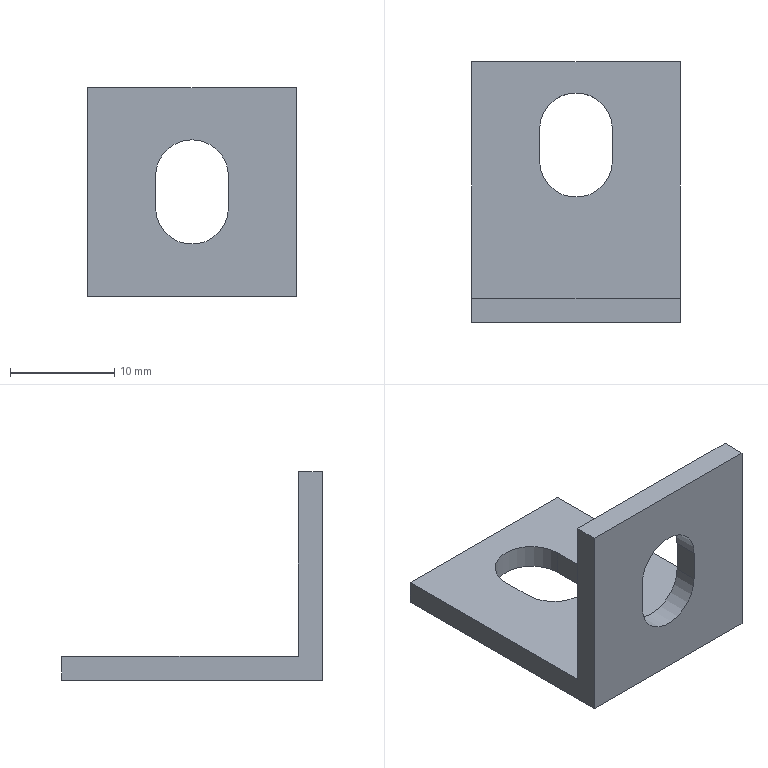Part | STEP file | Mirror BRACKET_0829_041_CRONWB29 | 1 solid | 17 faces | box 20 x 25 x 20 mm | volume 1691 mm3 | plane 12 | cylinder 5 | commonest cylinder face diameters 7 x5
STEP:
#1=CARTESIAN_POINT('',(0.,2.3,15.));
#2=VERTEX_POINT('',#1);
#3=CARTESIAN_POINT('',(-3.5,2.3,11.5));
#4=VERTEX_POINT('',#3);
#5=CARTESIAN_POINT('',(0.,2.3,11.5));
#6=DIRECTION('',(0.,-1.,0.));
#7=DIRECTION('',(0.,0.,1.));
#8=AXIS2_PLACEMENT_3D('',#5,#6,#7);
#9=CIRCLE('',#8,3.5);
#10=EDGE_CURVE('',#2,#4,#9,.T.);
#11=ORIENTED_EDGE('',*,*,#10,.F.);
#12=CARTESIAN_POINT('',(0.,0.,15.));
#13=VERTEX_POINT('',#12);
#14=CARTESIAN_POINT('',(0.,25.,15.));
#15=DIRECTION('',(0.,-1.,0.));
#16=VECTOR('',#15,1000.);
#17=LINE('',#14,#16);
#18=EDGE_CURVE('',#2,#13,#17,.T.);
#19=ORIENTED_EDGE('',*,*,#18,.T.);
#20=CARTESIAN_POINT('',(-3.5,0.,11.5));
#21=VERTEX_POINT('',#20);
#22=CARTESIAN_POINT('',(0.,0.,11.5));
#23=DIRECTION('',(0.,-1.,0.));
#24=DIRECTION('',(0.,0.,-1.));
#25=AXIS2_PLACEMENT_3D('',#22,#23,#24);
#26=CIRCLE('',#25,3.5);
#27=EDGE_CURVE('',#13,#21,#26,.T.);
#28=ORIENTED_EDGE('',*,*,#27,.T.);
#29=CARTESIAN_POINT('',(-3.5,25.,11.5));
#30=DIRECTION('',(0.,-1.,0.));
#31=VECTOR('',#30,1000.);
#32=LINE('',#29,#31);
#33=EDGE_CURVE('',#4,#21,#32,.T.);
#34=ORIENTED_EDGE('',*,*,#33,.F.);
#35=EDGE_LOOP('',(#11,#19,#28,#34));
#36=FACE_OUTER_BOUND('',#35,.T.);
#37=CARTESIAN_POINT('',(0.,25.,11.5));
#38=DIRECTION('',(0.,-1.,0.));
#39=DIRECTION('',(0.,0.,1.));
#40=AXIS2_PLACEMENT_3D('',#37,#38,#39);
#41=CYLINDRICAL_SURFACE('',#40,3.5);
#42=ADVANCED_FACE('',(#36),#41,.F.);
#43=CARTESIAN_POINT('',(-10.,0.,0.));
#44=VERTEX_POINT('',#43);
#45=CARTESIAN_POINT('',(-10.,0.,20.));
#46=VERTEX_POINT('',#45);
#47=CARTESIAN_POINT('',(-10.,0.,0.));
#48=DIRECTION('',(0.,0.,1.));
#49=VECTOR('',#48,1000.);
#50=LINE('',#47,#49);
#51=EDGE_CURVE('',#44,#46,#50,.T.);
#52=ORIENTED_EDGE('',*,*,#51,.F.);
#53=CARTESIAN_POINT('',(10.,0.,0.));
#54=VERTEX_POINT('',#53);
#55=CARTESIAN_POINT('',(10.,0.,0.));
#56=DIRECTION('',(-1.,0.,0.));
#57=VECTOR('',#56,1000.);
#58=LINE('',#55,#57);
#59=EDGE_CURVE('',#54,#44,#58,.T.);
#60=ORIENTED_EDGE('',*,*,#59,.F.);
#61=CARTESIAN_POINT('',(10.,0.,20.));
#62=VERTEX_POINT('',#61);
#63=CARTESIAN_POINT('',(10.,0.,0.));
#64=DIRECTION('',(0.,0.,1.));
#65=VECTOR('',#64,1000.);
#66=LINE('',#63,#65);
#67=EDGE_CURVE('',#54,#62,#66,.T.);
#68=ORIENTED_EDGE('',*,*,#67,.T.);
#69=CARTESIAN_POINT('',(10.,0.,20.));
#70=DIRECTION('',(-1.,0.,0.));
#71=VECTOR('',#70,1000.);
#72=LINE('',#69,#71);
#73=EDGE_CURVE('',#62,#46,#72,.T.);
#74=ORIENTED_EDGE('',*,*,#73,.T.);
#75=EDGE_LOOP('',(#52,#60,#68,#74));
#76=FACE_OUTER_BOUND('',#75,.T.);
#77=CARTESIAN_POINT('',(3.5,0.,11.5));
#78=VERTEX_POINT('',#77);
#79=CARTESIAN_POINT('',(0.,0.,11.5));
#80=DIRECTION('',(0.,-1.,0.));
#81=DIRECTION('',(0.,0.,-1.));
#82=AXIS2_PLACEMENT_3D('',#79,#80,#81);
#83=CIRCLE('',#82,3.5);
#84=EDGE_CURVE('',#78,#13,#83,.T.);
#85=ORIENTED_EDGE('',*,*,#84,.F.);
#86=CARTESIAN_POINT('',(3.5,0.,8.5));
#87=VERTEX_POINT('',#86);
#88=CARTESIAN_POINT('',(3.5,0.,11.5));
#89=DIRECTION('',(0.,0.,1.));
#90=VECTOR('',#89,1000.);
#91=LINE('',#88,#90);
#92=EDGE_CURVE('',#87,#78,#91,.T.);
#93=ORIENTED_EDGE('',*,*,#92,.F.);
#94=CARTESIAN_POINT('',(-3.5,0.,8.5));
#95=VERTEX_POINT('',#94);
#96=CARTESIAN_POINT('',(0.,0.,8.5));
#97=DIRECTION('',(0.,-1.,0.));
#98=DIRECTION('',(0.,0.,-1.));
#99=AXIS2_PLACEMENT_3D('',#96,#97,#98);
#100=CIRCLE('',#99,3.5);
#101=EDGE_CURVE('',#95,#87,#100,.T.);
#102=ORIENTED_EDGE('',*,*,#101,.F.);
#103=CARTESIAN_POINT('',(-3.5,0.,11.5));
#104=DIRECTION('',(0.,0.,-1.));
#105=VECTOR('',#104,1000.);
#106=LINE('',#103,#105);
#107=EDGE_CURVE('',#21,#95,#106,.T.);
#108=ORIENTED_EDGE('',*,*,#107,.F.);
#109=ORIENTED_EDGE('',*,*,#27,.F.);
#110=EDGE_LOOP('',(#85,#93,#102,#108,#109));
#111=FACE_BOUND('',#110,.T.);
#112=CARTESIAN_POINT('',(10.,0.,0.));
#113=DIRECTION('',(0.,1.,0.));
#114=DIRECTION('',(0.,0.,-1.));
#115=AXIS2_PLACEMENT_3D('',#112,#113,#114);
#116=PLANE('',#115);
#117=ADVANCED_FACE('',(#76,#111),#116,.F.);
#118=CARTESIAN_POINT('',(-10.,2.3,20.));
#119=VERTEX_POINT('',#118);
#120=CARTESIAN_POINT('',(-10.,2.3,2.3));
#121=VERTEX_POINT('',#120);
#122=CARTESIAN_POINT('',(-10.,2.3,20.));
#123=DIRECTION('',(0.,0.,-1.));
#124=VECTOR('',#123,1000.);
#125=LINE('',#122,#124);
#126=EDGE_CURVE('',#119,#121,#125,.T.);
#127=ORIENTED_EDGE('',*,*,#126,.F.);
#128=CARTESIAN_POINT('',(10.,2.3,20.));
#129=VERTEX_POINT('',#128);
#130=CARTESIAN_POINT('',(10.,2.3,20.));
#131=DIRECTION('',(-1.,0.,0.));
#132=VECTOR('',#131,1000.);
#133=LINE('',#130,#132);
#134=EDGE_CURVE('',#129,#119,#133,.T.);
#135=ORIENTED_EDGE('',*,*,#134,.F.);
#136=CARTESIAN_POINT('',(10.,2.3,2.3));
#137=VERTEX_POINT('',#136);
#138=CARTESIAN_POINT('',(10.,2.3,20.));
#139=DIRECTION('',(0.,0.,-1.));
#140=VECTOR('',#139,1000.);
#141=LINE('',#138,#140);
#142=EDGE_CURVE('',#129,#137,#141,.T.);
#143=ORIENTED_EDGE('',*,*,#142,.T.);
#144=CARTESIAN_POINT('',(10.,2.3,2.3));
#145=DIRECTION('',(-1.,0.,0.));
#146=VECTOR('',#145,1000.);
#147=LINE('',#144,#146);
#148=EDGE_CURVE('',#137,#121,#147,.T.);
#149=ORIENTED_EDGE('',*,*,#148,.T.);
#150=EDGE_LOOP('',(#127,#135,#143,#149));
#151=FACE_OUTER_BOUND('',#150,.T.);
#152=CARTESIAN_POINT('',(3.5,2.3,11.5));
#153=VERTEX_POINT('',#152);
#154=CARTESIAN_POINT('',(0.,2.3,11.5));
#155=DIRECTION('',(0.,-1.,0.));
#156=DIRECTION('',(0.,0.,1.));
#157=AXIS2_PLACEMENT_3D('',#154,#155,#156);
#158=CIRCLE('',#157,3.5);
#159=EDGE_CURVE('',#153,#2,#158,.T.);
#160=ORIENTED_EDGE('',*,*,#159,.T.);
#161=ORIENTED_EDGE('',*,*,#10,.T.);
#162=CARTESIAN_POINT('',(-3.5,2.3,8.5));
#163=VERTEX_POINT('',#162);
#164=CARTESIAN_POINT('',(-3.5,2.3,20.));
#165=DIRECTION('',(0.,0.,-1.));
#166=VECTOR('',#165,1000.);
#167=LINE('',#164,#166);
#168=EDGE_CURVE('',#4,#163,#167,.T.);
#169=ORIENTED_EDGE('',*,*,#168,.T.);
#170=CARTESIAN_POINT('',(3.5,2.3,8.5));
#171=VERTEX_POINT('',#170);
#172=CARTESIAN_POINT('',(0.,2.3,8.5));
#173=DIRECTION('',(0.,-1.,0.));
#174=DIRECTION('',(0.,0.,1.));
#175=AXIS2_PLACEMENT_3D('',#172,#173,#174);
#176=CIRCLE('',#175,3.5);
#177=EDGE_CURVE('',#163,#171,#176,.T.);
#178=ORIENTED_EDGE('',*,*,#177,.T.);
#179=CARTESIAN_POINT('',(3.5,2.3,20.));
#180=DIRECTION('',(0.,0.,1.));
#181=VECTOR('',#180,1000.);
#182=LINE('',#179,#181);
#183=EDGE_CURVE('',#171,#153,#182,.T.);
#184=ORIENTED_EDGE('',*,*,#183,.T.);
#185=EDGE_LOOP('',(#160,#161,#169,#178,#184));
#186=FACE_BOUND('',#185,.T.);
#187=CARTESIAN_POINT('',(10.,2.3,20.));
#188=DIRECTION('',(0.,-1.,0.));
#189=DIRECTION('',(0.,0.,1.));
#190=AXIS2_PLACEMENT_3D('',#187,#188,#189);
#191=PLANE('',#190);
#192=ADVANCED_FACE('',(#151,#186),#191,.F.);
#193=CARTESIAN_POINT('',(-10.,25.,2.3));
#194=VERTEX_POINT('',#193);
#195=CARTESIAN_POINT('',(-10.,25.,0.));
#196=VERTEX_POINT('',#195);
#197=CARTESIAN_POINT('',(-10.,25.,2.3));
#198=DIRECTION('',(0.,0.,-1.));
#199=VECTOR('',#198,1000.);
#200=LINE('',#197,#199);
#201=EDGE_CURVE('',#194,#196,#200,.T.);
#202=ORIENTED_EDGE('',*,*,#201,.F.);
#203=CARTESIAN_POINT('',(10.,25.,2.3));
#204=VERTEX_POINT('',#203);
#205=CARTESIAN_POINT('',(10.,25.,2.3));
#206=DIRECTION('',(-1.,0.,0.));
#207=VECTOR('',#206,1000.);
#208=LINE('',#205,#207);
#209=EDGE_CURVE('',#204,#194,#208,.T.);
#210=ORIENTED_EDGE('',*,*,#209,.F.);
#211=CARTESIAN_POINT('',(10.,25.,0.));
#212=VERTEX_POINT('',#211);
#213=CARTESIAN_POINT('',(10.,25.,2.3));
#214=DIRECTION('',(0.,0.,-1.));
#215=VECTOR('',#214,1000.);
#216=LINE('',#213,#215);
#217=EDGE_CURVE('',#204,#212,#216,.T.);
#218=ORIENTED_EDGE('',*,*,#217,.T.);
#219=CARTESIAN_POINT('',(10.,25.,0.));
#220=DIRECTION('',(-1.,0.,0.));
#221=VECTOR('',#220,1000.);
#222=LINE('',#219,#221);
#223=EDGE_CURVE('',#212,#196,#222,.T.);
#224=ORIENTED_EDGE('',*,*,#223,.T.);
#225=EDGE_LOOP('',(#202,#210,#218,#224));
#226=FACE_OUTER_BOUND('',#225,.T.);
#227=CARTESIAN_POINT('',(10.,25.,2.3));
#228=DIRECTION('',(0.,-1.,0.));
#229=DIRECTION('',(0.,0.,1.));
#230=AXIS2_PLACEMENT_3D('',#227,#228,#229);
#231=PLANE('',#230);
#232=ADVANCED_FACE('',(#226),#231,.F.);
#233=CARTESIAN_POINT('',(-3.5,18.5,0.));
#234=VERTEX_POINT('',#233);
#235=CARTESIAN_POINT('',(-3.5,15.5,0.));
#236=VERTEX_POINT('',#235);
#237=CARTESIAN_POINT('',(-3.5,18.5,0.));
#238=DIRECTION('',(0.,-1.,0.));
#239=VECTOR('',#238,1000.);
#240=LINE('',#237,#239);
#241=EDGE_CURVE('',#234,#236,#240,.T.);
#242=ORIENTED_EDGE('',*,*,#241,.T.);
#243=CARTESIAN_POINT('',(3.5,15.5,0.));
#244=VERTEX_POINT('',#243);
#245=CARTESIAN_POINT('',(0.,15.5,0.));
#246=DIRECTION('',(0.,0.,1.));
#247=DIRECTION('',(1.,0.,0.));
#248=AXIS2_PLACEMENT_3D('',#245,#246,#247);
#249=CIRCLE('',#248,3.5);
#250=EDGE_CURVE('',#236,#244,#249,.T.);
#251=ORIENTED_EDGE('',*,*,#250,.T.);
#252=CARTESIAN_POINT('',(3.5,18.5,0.));
#253=VERTEX_POINT('',#252);
#254=CARTESIAN_POINT('',(3.5,18.5,0.));
#255=DIRECTION('',(0.,1.,0.));
#256=VECTOR('',#255,1000.);
#257=LINE('',#254,#256);
#258=EDGE_CURVE('',#244,#253,#257,.T.);
#259=ORIENTED_EDGE('',*,*,#258,.T.);
#260=CARTESIAN_POINT('',(0.,18.5,0.));
#261=DIRECTION('',(0.,0.,1.));
#262=DIRECTION('',(1.,0.,0.));
#263=AXIS2_PLACEMENT_3D('',#260,#261,#262);
#264=CIRCLE('',#263,3.5);
#265=EDGE_CURVE('',#253,#234,#264,.T.);
#266=ORIENTED_EDGE('',*,*,#265,.T.);
#267=EDGE_LOOP('',(#242,#251,#259,#266));
#268=FACE_BOUND('',#267,.T.);
#269=CARTESIAN_POINT('',(-10.,25.,0.));
#270=DIRECTION('',(0.,-1.,0.));
#271=VECTOR('',#270,1000.);
#272=LINE('',#269,#271);
#273=EDGE_CURVE('',#196,#44,#272,.T.);
#274=ORIENTED_EDGE('',*,*,#273,.F.);
#275=ORIENTED_EDGE('',*,*,#223,.F.);
#276=CARTESIAN_POINT('',(10.,25.,0.));
#277=DIRECTION('',(0.,-1.,0.));
#278=VECTOR('',#277,1000.);
#279=LINE('',#276,#278);
#280=EDGE_CURVE('',#212,#54,#279,.T.);
#281=ORIENTED_EDGE('',*,*,#280,.T.);
#282=ORIENTED_EDGE('',*,*,#59,.T.);
#283=EDGE_LOOP('',(#274,#275,#281,#282));
#284=FACE_OUTER_BOUND('',#283,.T.);
#285=CARTESIAN_POINT('',(10.,25.,0.));
#286=DIRECTION('',(0.,0.,1.));
#287=DIRECTION('',(0.,1.,0.));
#288=AXIS2_PLACEMENT_3D('',#285,#286,#287);
#289=PLANE('',#288);
#290=ADVANCED_FACE('',(#268,#284),#289,.F.);
#291=CARTESIAN_POINT('',(-10.,0.,20.));
#292=DIRECTION('',(0.,1.,0.));
#293=VECTOR('',#292,1000.);
#294=LINE('',#291,#293);
#295=EDGE_CURVE('',#46,#119,#294,.T.);
#296=ORIENTED_EDGE('',*,*,#295,.F.);
#297=ORIENTED_EDGE('',*,*,#73,.F.);
#298=CARTESIAN_POINT('',(10.,0.,20.));
#299=DIRECTION('',(0.,1.,0.));
#300=VECTOR('',#299,1000.);
#301=LINE('',#298,#300);
#302=EDGE_CURVE('',#62,#129,#301,.T.);
#303=ORIENTED_EDGE('',*,*,#302,.T.);
#304=ORIENTED_EDGE('',*,*,#134,.T.);
#305=EDGE_LOOP('',(#296,#297,#303,#304));
#306=FACE_OUTER_BOUND('',#305,.T.);
#307=CARTESIAN_POINT('',(10.,0.,20.));
#308=DIRECTION('',(0.,0.,-1.));
#309=DIRECTION('',(1.,0.,0.));
#310=AXIS2_PLACEMENT_3D('',#307,#308,#309);
#311=PLANE('',#310);
#312=ADVANCED_FACE('',(#306),#311,.F.);
#313=CARTESIAN_POINT('',(3.5,15.5,2.3));
#314=VERTEX_POINT('',#313);
#315=CARTESIAN_POINT('',(3.5,18.5,2.3));
#316=VERTEX_POINT('',#315);
#317=CARTESIAN_POINT('',(3.5,2.3,2.3));
#318=DIRECTION('',(0.,1.,0.));
#319=VECTOR('',#318,1000.);
#320=LINE('',#317,#319);
#321=EDGE_CURVE('',#314,#316,#320,.T.);
#322=ORIENTED_EDGE('',*,*,#321,.F.);
#323=CARTESIAN_POINT('',(-3.5,15.5,2.3));
#324=VERTEX_POINT('',#323);
#325=CARTESIAN_POINT('',(0.,15.5,2.3));
#326=DIRECTION('',(0.,0.,1.));
#327=DIRECTION('',(1.,0.,0.));
#328=AXIS2_PLACEMENT_3D('',#325,#326,#327);
#329=CIRCLE('',#328,3.5);
#330=EDGE_CURVE('',#324,#314,#329,.T.);
#331=ORIENTED_EDGE('',*,*,#330,.F.);
#332=CARTESIAN_POINT('',(-3.5,18.5,2.3));
#333=VERTEX_POINT('',#332);
#334=CARTESIAN_POINT('',(-3.5,2.3,2.3));
#335=DIRECTION('',(0.,-1.,0.));
#336=VECTOR('',#335,1000.);
#337=LINE('',#334,#336);
#338=EDGE_CURVE('',#333,#324,#337,.T.);
#339=ORIENTED_EDGE('',*,*,#338,.F.);
#340=CARTESIAN_POINT('',(0.,18.5,2.3));
#341=DIRECTION('',(0.,0.,1.));
#342=DIRECTION('',(1.,0.,0.));
#343=AXIS2_PLACEMENT_3D('',#340,#341,#342);
#344=CIRCLE('',#343,3.5);
#345=EDGE_CURVE('',#316,#333,#344,.T.);
#346=ORIENTED_EDGE('',*,*,#345,.F.);
#347=EDGE_LOOP('',(#322,#331,#339,#346));
#348=FACE_BOUND('',#347,.T.);
#349=CARTESIAN_POINT('',(-10.,2.3,2.3));
#350=DIRECTION('',(0.,1.,0.));
#351=VECTOR('',#350,1000.);
#352=LINE('',#349,#351);
#353=EDGE_CURVE('',#121,#194,#352,.T.);
#354=ORIENTED_EDGE('',*,*,#353,.F.);
#355=ORIENTED_EDGE('',*,*,#148,.F.);
#356=CARTESIAN_POINT('',(10.,2.3,2.3));
#357=DIRECTION('',(0.,1.,0.));
#358=VECTOR('',#357,1000.);
#359=LINE('',#356,#358);
#360=EDGE_CURVE('',#137,#204,#359,.T.);
#361=ORIENTED_EDGE('',*,*,#360,.T.);
#362=ORIENTED_EDGE('',*,*,#209,.T.);
#363=EDGE_LOOP('',(#354,#355,#361,#362));
#364=FACE_OUTER_BOUND('',#363,.T.);
#365=CARTESIAN_POINT('',(10.,2.3,2.3));
#366=DIRECTION('',(0.,0.,-1.));
#367=DIRECTION('',(1.,0.,0.));
#368=AXIS2_PLACEMENT_3D('',#365,#366,#367);
#369=PLANE('',#368);
#370=ADVANCED_FACE('',(#348,#364),#369,.F.);
#371=ORIENTED_EDGE('',*,*,#217,.F.);
#372=ORIENTED_EDGE('',*,*,#360,.F.);
#373=ORIENTED_EDGE('',*,*,#142,.F.);
#374=ORIENTED_EDGE('',*,*,#302,.F.);
#375=ORIENTED_EDGE('',*,*,#67,.F.);
#376=ORIENTED_EDGE('',*,*,#280,.F.);
#377=EDGE_LOOP('',(#371,#372,#373,#374,#375,#376));
#378=FACE_OUTER_BOUND('',#377,.T.);
#379=CARTESIAN_POINT('',(10.,0.,0.));
#380=DIRECTION('',(1.,0.,0.));
#381=DIRECTION('',(0.,0.,1.));
#382=AXIS2_PLACEMENT_3D('',#379,#380,#381);
#383=PLANE('',#382);
#384=ADVANCED_FACE('',(#378),#383,.T.);
#385=ORIENTED_EDGE('',*,*,#201,.T.);
#386=ORIENTED_EDGE('',*,*,#273,.T.);
#387=ORIENTED_EDGE('',*,*,#51,.T.);
#388=ORIENTED_EDGE('',*,*,#295,.T.);
#389=ORIENTED_EDGE('',*,*,#126,.T.);
#390=ORIENTED_EDGE('',*,*,#353,.T.);
#391=EDGE_LOOP('',(#385,#386,#387,#388,#389,#390));
#392=FACE_OUTER_BOUND('',#391,.T.);
#393=CARTESIAN_POINT('',(-10.,0.,0.));
#394=DIRECTION('',(1.,0.,0.));
#395=DIRECTION('',(0.,0.,1.));
#396=AXIS2_PLACEMENT_3D('',#393,#394,#395);
#397=PLANE('',#396);
#398=ADVANCED_FACE('',(#392),#397,.F.);
#399=CARTESIAN_POINT('',(3.5,18.5,20.));
#400=DIRECTION('',(0.,0.,-1.));
#401=VECTOR('',#400,1000.);
#402=LINE('',#399,#401);
#403=EDGE_CURVE('',#316,#253,#402,.T.);
#404=ORIENTED_EDGE('',*,*,#403,.F.);
#405=ORIENTED_EDGE('',*,*,#345,.T.);
#406=CARTESIAN_POINT('',(-3.5,18.5,20.));
#407=DIRECTION('',(0.,0.,-1.));
#408=VECTOR('',#407,1000.);
#409=LINE('',#406,#408);
#410=EDGE_CURVE('',#333,#234,#409,.T.);
#411=ORIENTED_EDGE('',*,*,#410,.T.);
#412=ORIENTED_EDGE('',*,*,#265,.F.);
#413=EDGE_LOOP('',(#404,#405,#411,#412));
#414=FACE_OUTER_BOUND('',#413,.T.);
#415=CARTESIAN_POINT('',(0.,18.5,20.));
#416=DIRECTION('',(0.,0.,-1.));
#417=DIRECTION('',(1.,0.,0.));
#418=AXIS2_PLACEMENT_3D('',#415,#416,#417);
#419=CYLINDRICAL_SURFACE('',#418,3.5);
#420=ADVANCED_FACE('',(#414),#419,.F.);
#421=CARTESIAN_POINT('',(3.5,15.5,20.));
#422=DIRECTION('',(0.,0.,-1.));
#423=VECTOR('',#422,1000.);
#424=LINE('',#421,#423);
#425=EDGE_CURVE('',#314,#244,#424,.T.);
#426=ORIENTED_EDGE('',*,*,#425,.F.);
#427=ORIENTED_EDGE('',*,*,#321,.T.);
#428=ORIENTED_EDGE('',*,*,#403,.T.);
#429=ORIENTED_EDGE('',*,*,#258,.F.);
#430=EDGE_LOOP('',(#426,#427,#428,#429));
#431=FACE_OUTER_BOUND('',#430,.T.);
#432=CARTESIAN_POINT('',(3.5,18.5,20.));
#433=DIRECTION('',(1.,0.,0.));
#434=DIRECTION('',(0.,0.,1.));
#435=AXIS2_PLACEMENT_3D('',#432,#433,#434);
#436=PLANE('',#435);
#437=ADVANCED_FACE('',(#431),#436,.F.);
#438=CARTESIAN_POINT('',(-3.5,15.5,20.));
#439=DIRECTION('',(0.,0.,-1.));
#440=VECTOR('',#439,1000.);
#441=LINE('',#438,#440);
#442=EDGE_CURVE('',#324,#236,#441,.T.);
#443=ORIENTED_EDGE('',*,*,#442,.F.);
#444=ORIENTED_EDGE('',*,*,#330,.T.);
#445=ORIENTED_EDGE('',*,*,#425,.T.);
#446=ORIENTED_EDGE('',*,*,#250,.F.);
#447=EDGE_LOOP('',(#443,#444,#445,#446));
#448=FACE_OUTER_BOUND('',#447,.T.);
#449=CARTESIAN_POINT('',(0.,15.5,20.));
#450=DIRECTION('',(0.,0.,-1.));
#451=DIRECTION('',(1.,0.,0.));
#452=AXIS2_PLACEMENT_3D('',#449,#450,#451);
#453=CYLINDRICAL_SURFACE('',#452,3.5);
#454=ADVANCED_FACE('',(#448),#453,.F.);
#455=ORIENTED_EDGE('',*,*,#410,.F.);
#456=ORIENTED_EDGE('',*,*,#338,.T.);
#457=ORIENTED_EDGE('',*,*,#442,.T.);
#458=ORIENTED_EDGE('',*,*,#241,.F.);
#459=EDGE_LOOP('',(#455,#456,#457,#458));
#460=FACE_OUTER_BOUND('',#459,.T.);
#461=CARTESIAN_POINT('',(-3.5,18.5,20.));
#462=DIRECTION('',(-1.,0.,0.));
#463=DIRECTION('',(0.,0.,-1.));
#464=AXIS2_PLACEMENT_3D('',#461,#462,#463);
#465=PLANE('',#464);
#466=ADVANCED_FACE('',(#460),#465,.F.);
#467=ORIENTED_EDGE('',*,*,#18,.F.);
#468=ORIENTED_EDGE('',*,*,#159,.F.);
#469=CARTESIAN_POINT('',(3.5,25.,11.5));
#470=DIRECTION('',(0.,-1.,0.));
#471=VECTOR('',#470,1000.);
#472=LINE('',#469,#471);
#473=EDGE_CURVE('',#153,#78,#472,.T.);
#474=ORIENTED_EDGE('',*,*,#473,.T.);
#475=ORIENTED_EDGE('',*,*,#84,.T.);
#476=EDGE_LOOP('',(#467,#468,#474,#475));
#477=FACE_OUTER_BOUND('',#476,.T.);
#478=CARTESIAN_POINT('',(0.,25.,11.5));
#479=DIRECTION('',(0.,-1.,0.));
#480=DIRECTION('',(0.,0.,1.));
#481=AXIS2_PLACEMENT_3D('',#478,#479,#480);
#482=CYLINDRICAL_SURFACE('',#481,3.5);
#483=ADVANCED_FACE('',(#477),#482,.F.);
#484=ORIENTED_EDGE('',*,*,#168,.F.);
#485=ORIENTED_EDGE('',*,*,#33,.T.);
#486=ORIENTED_EDGE('',*,*,#107,.T.);
#487=CARTESIAN_POINT('',(-3.5,25.,8.5));
#488=DIRECTION('',(0.,-1.,0.));
#489=VECTOR('',#488,1000.);
#490=LINE('',#487,#489);
#491=EDGE_CURVE('',#163,#95,#490,.T.);
#492=ORIENTED_EDGE('',*,*,#491,.F.);
#493=EDGE_LOOP('',(#484,#485,#486,#492));
#494=FACE_OUTER_BOUND('',#493,.T.);
#495=CARTESIAN_POINT('',(-3.5,25.,11.5));
#496=DIRECTION('',(1.,0.,0.));
#497=DIRECTION('',(0.,0.,1.));
#498=AXIS2_PLACEMENT_3D('',#495,#496,#497);
#499=PLANE('',#498);
#500=ADVANCED_FACE('',(#494),#499,.T.);
#501=ORIENTED_EDGE('',*,*,#177,.F.);
#502=ORIENTED_EDGE('',*,*,#491,.T.);
#503=ORIENTED_EDGE('',*,*,#101,.T.);
#504=CARTESIAN_POINT('',(3.5,25.,8.5));
#505=DIRECTION('',(0.,-1.,0.));
#506=VECTOR('',#505,1000.);
#507=LINE('',#504,#506);
#508=EDGE_CURVE('',#171,#87,#507,.T.);
#509=ORIENTED_EDGE('',*,*,#508,.F.);
#510=EDGE_LOOP('',(#501,#502,#503,#509));
#511=FACE_OUTER_BOUND('',#510,.T.);
#512=CARTESIAN_POINT('',(0.,25.,8.5));
#513=DIRECTION('',(0.,-1.,0.));
#514=DIRECTION('',(0.,0.,1.));
#515=AXIS2_PLACEMENT_3D('',#512,#513,#514);
#516=CYLINDRICAL_SURFACE('',#515,3.5);
#517=ADVANCED_FACE('',(#511),#516,.F.);
#518=ORIENTED_EDGE('',*,*,#183,.F.);
#519=ORIENTED_EDGE('',*,*,#508,.T.);
#520=ORIENTED_EDGE('',*,*,#92,.T.);
#521=ORIENTED_EDGE('',*,*,#473,.F.);
#522=EDGE_LOOP('',(#518,#519,#520,#521));
#523=FACE_OUTER_BOUND('',#522,.T.);
#524=CARTESIAN_POINT('',(3.5,25.,11.5));
#525=DIRECTION('',(-1.,0.,0.));
#526=DIRECTION('',(0.,0.,-1.));
#527=AXIS2_PLACEMENT_3D('',#524,#525,#526);
#528=PLANE('',#527);
#529=ADVANCED_FACE('',(#523),#528,.T.);
#530=CLOSED_SHELL('',(#42,#117,#192,#232,#290,#312,#370,#384,#398,#420,#437,#454,#466,#483,#500,#517,#529));
#531=MANIFOLD_SOLID_BREP('',#530);
#532=CARTESIAN_POINT('',(0.,0.,0.));
#533=DIRECTION('',(0.,0.,1.));
#534=DIRECTION('',(1.,0.,0.));
#535=AXIS2_PLACEMENT_3D('',#532,#533,#534);
#536=(LENGTH_UNIT()NAMED_UNIT(*)SI_UNIT(.MILLI.,.METRE.));
#537=UNCERTAINTY_MEASURE_WITH_UNIT(LENGTH_MEASURE(0.00001),#536,'','');
#538=(NAMED_UNIT(*)PLANE_ANGLE_UNIT()SI_UNIT($,.RADIAN.));
#539=(NAMED_UNIT(*)SI_UNIT($,.STERADIAN.)SOLID_ANGLE_UNIT());
#540=(GEOMETRIC_REPRESENTATION_CONTEXT(3)GLOBAL_UNCERTAINTY_ASSIGNED_CONTEXT((#537))GLOBAL_UNIT_ASSIGNED_CONTEXT((#536,#538,#539))REPRESENTATION_CONTEXT('',''));
#541=ADVANCED_BREP_SHAPE_REPRESENTATION('',(#531,#535),#540);